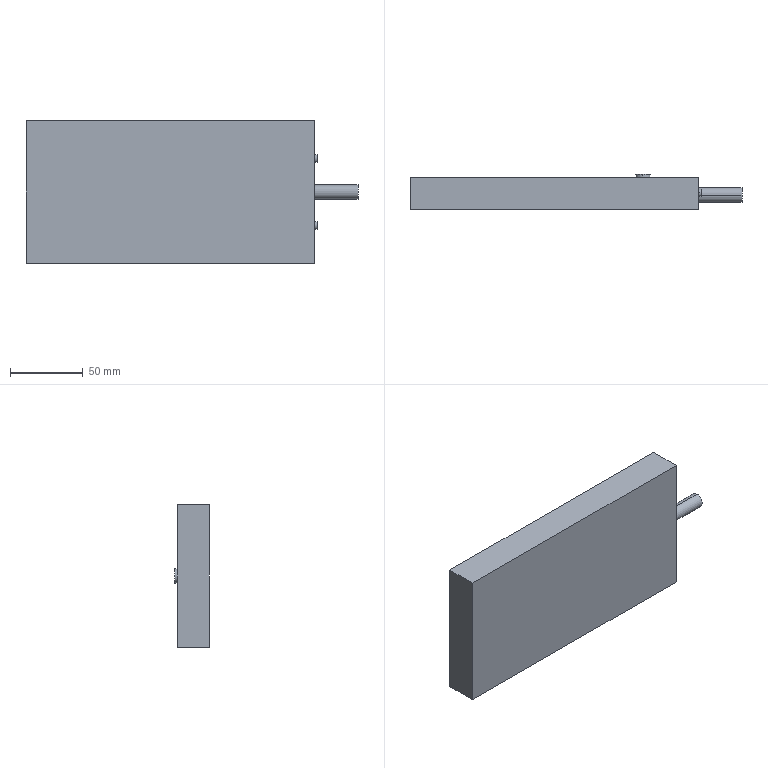Part | SolidWorks | features ICE 3, Extrusion 1 | 1 solid | 18 faces | box 228 x 24 x 98 mm | volume 429480 mm3 | plane 10 | cylinder 8 | commonest cylinder face diameters 5 x4 10 x4
STEP:
#1=CARTESIAN_POINT('',(101.,11.325,20.5));
#2=VERTEX_POINT('',#1);
#3=CARTESIAN_POINT('',(101.,11.325,25.5));
#4=VERTEX_POINT('',#3);
#5=CARTESIAN_POINT('',(101.,11.325,23.));
#6=DIRECTION('',(1.,0.,0.));
#7=DIRECTION('',(0.,0.,-1.));
#8=AXIS2_PLACEMENT_3D('',#5,#6,#7);
#9=CIRCLE('',#8,2.5);
#10=EDGE_CURVE('',#2,#4,#9,.T.);
#11=ORIENTED_EDGE('',*,*,#10,.F.);
#12=CARTESIAN_POINT('',(99.,11.325,20.5));
#13=VERTEX_POINT('',#12);
#14=CARTESIAN_POINT('',(101.,11.325,20.5));
#15=DIRECTION('',(-1.,0.,0.));
#16=VECTOR('',#15,1000.);
#17=LINE('',#14,#16);
#18=EDGE_CURVE('',#2,#13,#17,.T.);
#19=ORIENTED_EDGE('',*,*,#18,.T.);
#20=CARTESIAN_POINT('',(99.,11.325,25.5));
#21=VERTEX_POINT('',#20);
#22=CARTESIAN_POINT('',(99.,11.325,23.));
#23=DIRECTION('',(1.,0.,0.));
#24=DIRECTION('',(0.,0.,1.));
#25=AXIS2_PLACEMENT_3D('',#22,#23,#24);
#26=CIRCLE('',#25,2.5);
#27=EDGE_CURVE('',#13,#21,#26,.T.);
#28=ORIENTED_EDGE('',*,*,#27,.T.);
#29=CARTESIAN_POINT('',(101.,11.325,25.5));
#30=DIRECTION('',(-1.,0.,0.));
#31=VECTOR('',#30,1000.);
#32=LINE('',#29,#31);
#33=EDGE_CURVE('',#4,#21,#32,.T.);
#34=ORIENTED_EDGE('',*,*,#33,.F.);
#35=EDGE_LOOP('',(#11,#19,#28,#34));
#36=FACE_OUTER_BOUND('',#35,.T.);
#37=CARTESIAN_POINT('',(101.,11.325,23.));
#38=DIRECTION('',(-1.,0.,0.));
#39=DIRECTION('',(0.,0.,1.));
#40=AXIS2_PLACEMENT_3D('',#37,#38,#39);
#41=CYLINDRICAL_SURFACE('',#40,2.5);
#42=ADVANCED_FACE('',(#36),#41,.T.);
#43=CARTESIAN_POINT('',(101.,10.331,-25.5));
#44=VERTEX_POINT('',#43);
#45=CARTESIAN_POINT('',(101.,10.331,-20.5));
#46=VERTEX_POINT('',#45);
#47=CARTESIAN_POINT('',(101.,10.331,-23.));
#48=DIRECTION('',(1.,0.,0.));
#49=DIRECTION('',(0.,0.,-1.));
#50=AXIS2_PLACEMENT_3D('',#47,#48,#49);
#51=CIRCLE('',#50,2.5);
#52=EDGE_CURVE('',#44,#46,#51,.T.);
#53=ORIENTED_EDGE('',*,*,#52,.F.);
#54=CARTESIAN_POINT('',(99.,10.331,-25.5));
#55=VERTEX_POINT('',#54);
#56=CARTESIAN_POINT('',(101.,10.331,-25.5));
#57=DIRECTION('',(-1.,0.,0.));
#58=VECTOR('',#57,1000.);
#59=LINE('',#56,#58);
#60=EDGE_CURVE('',#44,#55,#59,.T.);
#61=ORIENTED_EDGE('',*,*,#60,.T.);
#62=CARTESIAN_POINT('',(99.,10.331,-20.5));
#63=VERTEX_POINT('',#62);
#64=CARTESIAN_POINT('',(99.,10.331,-23.));
#65=DIRECTION('',(1.,0.,0.));
#66=DIRECTION('',(0.,0.,1.));
#67=AXIS2_PLACEMENT_3D('',#64,#65,#66);
#68=CIRCLE('',#67,2.5);
#69=EDGE_CURVE('',#55,#63,#68,.T.);
#70=ORIENTED_EDGE('',*,*,#69,.T.);
#71=CARTESIAN_POINT('',(101.,10.331,-20.5));
#72=DIRECTION('',(-1.,0.,0.));
#73=VECTOR('',#72,1000.);
#74=LINE('',#71,#73);
#75=EDGE_CURVE('',#46,#63,#74,.T.);
#76=ORIENTED_EDGE('',*,*,#75,.F.);
#77=EDGE_LOOP('',(#53,#61,#70,#76));
#78=FACE_OUTER_BOUND('',#77,.T.);
#79=CARTESIAN_POINT('',(101.,10.331,-23.));
#80=DIRECTION('',(-1.,0.,0.));
#81=DIRECTION('',(0.,0.,1.));
#82=AXIS2_PLACEMENT_3D('',#79,#80,#81);
#83=CYLINDRICAL_SURFACE('',#82,2.5);
#84=ADVANCED_FACE('',(#78),#83,.T.);
#85=CARTESIAN_POINT('',(61.,24.,5.));
#86=VERTEX_POINT('',#85);
#87=CARTESIAN_POINT('',(61.,24.,-5.));
#88=VERTEX_POINT('',#87);
#89=CARTESIAN_POINT('',(61.,24.,0.));
#90=DIRECTION('',(0.,1.,0.));
#91=DIRECTION('',(0.,0.,1.));
#92=AXIS2_PLACEMENT_3D('',#89,#90,#91);
#93=CIRCLE('',#92,5.);
#94=EDGE_CURVE('',#86,#88,#93,.T.);
#95=ORIENTED_EDGE('',*,*,#94,.F.);
#96=CARTESIAN_POINT('',(61.,22.,5.));
#97=VERTEX_POINT('',#96);
#98=CARTESIAN_POINT('',(61.,24.,5.));
#99=DIRECTION('',(0.,-1.,0.));
#100=VECTOR('',#99,1000.);
#101=LINE('',#98,#100);
#102=EDGE_CURVE('',#86,#97,#101,.T.);
#103=ORIENTED_EDGE('',*,*,#102,.T.);
#104=CARTESIAN_POINT('',(61.,22.,-5.));
#105=VERTEX_POINT('',#104);
#106=CARTESIAN_POINT('',(61.,22.,0.));
#107=DIRECTION('',(0.,1.,0.));
#108=DIRECTION('',(0.,0.,-1.));
#109=AXIS2_PLACEMENT_3D('',#106,#107,#108);
#110=CIRCLE('',#109,5.);
#111=EDGE_CURVE('',#97,#105,#110,.T.);
#112=ORIENTED_EDGE('',*,*,#111,.T.);
#113=CARTESIAN_POINT('',(61.,24.,-5.));
#114=DIRECTION('',(0.,-1.,0.));
#115=VECTOR('',#114,1000.);
#116=LINE('',#113,#115);
#117=EDGE_CURVE('',#88,#105,#116,.T.);
#118=ORIENTED_EDGE('',*,*,#117,.F.);
#119=EDGE_LOOP('',(#95,#103,#112,#118));
#120=FACE_OUTER_BOUND('',#119,.T.);
#121=CARTESIAN_POINT('',(61.,24.,0.));
#122=DIRECTION('',(0.,-1.,0.));
#123=DIRECTION('',(0.,0.,-1.));
#124=AXIS2_PLACEMENT_3D('',#121,#122,#123);
#125=CYLINDRICAL_SURFACE('',#124,5.);
#126=ADVANCED_FACE('',(#120),#125,.T.);
#127=CARTESIAN_POINT('',(129.,9.76,-5.));
#128=VERTEX_POINT('',#127);
#129=CARTESIAN_POINT('',(129.,9.76,5.));
#130=VERTEX_POINT('',#129);
#131=CARTESIAN_POINT('',(129.,9.76,0.));
#132=DIRECTION('',(1.,0.,0.));
#133=DIRECTION('',(0.,0.,-1.));
#134=AXIS2_PLACEMENT_3D('',#131,#132,#133);
#135=CIRCLE('',#134,5.);
#136=EDGE_CURVE('',#128,#130,#135,.T.);
#137=ORIENTED_EDGE('',*,*,#136,.F.);
#138=CARTESIAN_POINT('',(99.,9.76,-5.));
#139=VERTEX_POINT('',#138);
#140=CARTESIAN_POINT('',(129.,9.76,-5.));
#141=DIRECTION('',(-1.,0.,0.));
#142=VECTOR('',#141,1000.);
#143=LINE('',#140,#142);
#144=EDGE_CURVE('',#128,#139,#143,.T.);
#145=ORIENTED_EDGE('',*,*,#144,.T.);
#146=CARTESIAN_POINT('',(99.,9.76,5.));
#147=VERTEX_POINT('',#146);
#148=CARTESIAN_POINT('',(99.,9.76,0.));
#149=DIRECTION('',(1.,0.,0.));
#150=DIRECTION('',(0.,0.,1.));
#151=AXIS2_PLACEMENT_3D('',#148,#149,#150);
#152=CIRCLE('',#151,5.);
#153=EDGE_CURVE('',#139,#147,#152,.T.);
#154=ORIENTED_EDGE('',*,*,#153,.T.);
#155=CARTESIAN_POINT('',(129.,9.76,5.));
#156=DIRECTION('',(-1.,0.,0.));
#157=VECTOR('',#156,1000.);
#158=LINE('',#155,#157);
#159=EDGE_CURVE('',#130,#147,#158,.T.);
#160=ORIENTED_EDGE('',*,*,#159,.F.);
#161=EDGE_LOOP('',(#137,#145,#154,#160));
#162=FACE_OUTER_BOUND('',#161,.T.);
#163=CARTESIAN_POINT('',(129.,9.76,0.));
#164=DIRECTION('',(-1.,0.,0.));
#165=DIRECTION('',(0.,0.,1.));
#166=AXIS2_PLACEMENT_3D('',#163,#164,#165);
#167=CYLINDRICAL_SURFACE('',#166,5.);
#168=ADVANCED_FACE('',(#162),#167,.T.);
#169=CARTESIAN_POINT('',(99.,11.325,23.));
#170=DIRECTION('',(1.,0.,0.));
#171=DIRECTION('',(0.,0.,1.));
#172=AXIS2_PLACEMENT_3D('',#169,#170,#171);
#173=CIRCLE('',#172,2.5);
#174=EDGE_CURVE('',#21,#13,#173,.T.);
#175=ORIENTED_EDGE('',*,*,#174,.F.);
#176=ORIENTED_EDGE('',*,*,#27,.F.);
#177=EDGE_LOOP('',(#175,#176));
#178=FACE_BOUND('',#177,.T.);
#179=CARTESIAN_POINT('',(99.,10.331,-23.));
#180=DIRECTION('',(1.,0.,0.));
#181=DIRECTION('',(0.,0.,1.));
#182=AXIS2_PLACEMENT_3D('',#179,#180,#181);
#183=CIRCLE('',#182,2.5);
#184=EDGE_CURVE('',#63,#55,#183,.T.);
#185=ORIENTED_EDGE('',*,*,#184,.F.);
#186=ORIENTED_EDGE('',*,*,#69,.F.);
#187=EDGE_LOOP('',(#185,#186));
#188=FACE_BOUND('',#187,.T.);
#189=CARTESIAN_POINT('',(99.,9.76,0.));
#190=DIRECTION('',(1.,0.,0.));
#191=DIRECTION('',(0.,0.,1.));
#192=AXIS2_PLACEMENT_3D('',#189,#190,#191);
#193=CIRCLE('',#192,5.);
#194=EDGE_CURVE('',#147,#139,#193,.T.);
#195=ORIENTED_EDGE('',*,*,#194,.F.);
#196=ORIENTED_EDGE('',*,*,#153,.F.);
#197=EDGE_LOOP('',(#195,#196));
#198=FACE_BOUND('',#197,.T.);
#199=CARTESIAN_POINT('',(99.,0.,49.));
#200=VERTEX_POINT('',#199);
#201=CARTESIAN_POINT('',(99.,0.,-49.));
#202=VERTEX_POINT('',#201);
#203=CARTESIAN_POINT('',(99.,0.,49.));
#204=DIRECTION('',(0.,0.,-1.));
#205=VECTOR('',#204,1000.);
#206=LINE('',#203,#205);
#207=EDGE_CURVE('',#200,#202,#206,.T.);
#208=ORIENTED_EDGE('',*,*,#207,.T.);
#209=CARTESIAN_POINT('',(99.,22.,-49.));
#210=VERTEX_POINT('',#209);
#211=CARTESIAN_POINT('',(99.,22.,-49.));
#212=DIRECTION('',(0.,-1.,0.));
#213=VECTOR('',#212,1000.);
#214=LINE('',#211,#213);
#215=EDGE_CURVE('',#210,#202,#214,.T.);
#216=ORIENTED_EDGE('',*,*,#215,.F.);
#217=CARTESIAN_POINT('',(99.,22.,49.));
#218=VERTEX_POINT('',#217);
#219=CARTESIAN_POINT('',(99.,22.,49.));
#220=DIRECTION('',(0.,0.,-1.));
#221=VECTOR('',#220,1000.);
#222=LINE('',#219,#221);
#223=EDGE_CURVE('',#218,#210,#222,.T.);
#224=ORIENTED_EDGE('',*,*,#223,.F.);
#225=CARTESIAN_POINT('',(99.,22.,49.));
#226=DIRECTION('',(0.,-1.,0.));
#227=VECTOR('',#226,1000.);
#228=LINE('',#225,#227);
#229=EDGE_CURVE('',#218,#200,#228,.T.);
#230=ORIENTED_EDGE('',*,*,#229,.T.);
#231=EDGE_LOOP('',(#208,#216,#224,#230));
#232=FACE_OUTER_BOUND('',#231,.T.);
#233=CARTESIAN_POINT('',(99.,22.,49.));
#234=DIRECTION('',(-1.,0.,0.));
#235=DIRECTION('',(0.,0.,1.));
#236=AXIS2_PLACEMENT_3D('',#233,#234,#235);
#237=PLANE('',#236);
#238=ADVANCED_FACE('',(#178,#188,#198,#232),#237,.F.);
#239=CARTESIAN_POINT('',(-99.,0.,-49.));
#240=VERTEX_POINT('',#239);
#241=CARTESIAN_POINT('',(-99.,0.,-49.));
#242=DIRECTION('',(-1.,0.,0.));
#243=VECTOR('',#242,1000.);
#244=LINE('',#241,#243);
#245=EDGE_CURVE('',#202,#240,#244,.T.);
#246=ORIENTED_EDGE('',*,*,#245,.T.);
#247=CARTESIAN_POINT('',(-99.,22.,-49.));
#248=VERTEX_POINT('',#247);
#249=CARTESIAN_POINT('',(-99.,22.,-49.));
#250=DIRECTION('',(0.,-1.,0.));
#251=VECTOR('',#250,1000.);
#252=LINE('',#249,#251);
#253=EDGE_CURVE('',#248,#240,#252,.T.);
#254=ORIENTED_EDGE('',*,*,#253,.F.);
#255=CARTESIAN_POINT('',(-99.,22.,-49.));
#256=DIRECTION('',(-1.,0.,0.));
#257=VECTOR('',#256,1000.);
#258=LINE('',#255,#257);
#259=EDGE_CURVE('',#210,#248,#258,.T.);
#260=ORIENTED_EDGE('',*,*,#259,.F.);
#261=ORIENTED_EDGE('',*,*,#215,.T.);
#262=EDGE_LOOP('',(#246,#254,#260,#261));
#263=FACE_OUTER_BOUND('',#262,.T.);
#264=CARTESIAN_POINT('',(-99.,22.,-49.));
#265=DIRECTION('',(0.,0.,1.));
#266=DIRECTION('',(1.,0.,0.));
#267=AXIS2_PLACEMENT_3D('',#264,#265,#266);
#268=PLANE('',#267);
#269=ADVANCED_FACE('',(#263),#268,.F.);
#270=CARTESIAN_POINT('',(-99.,0.,49.));
#271=VERTEX_POINT('',#270);
#272=CARTESIAN_POINT('',(-99.,0.,49.));
#273=DIRECTION('',(0.,0.,1.));
#274=VECTOR('',#273,1000.);
#275=LINE('',#272,#274);
#276=EDGE_CURVE('',#240,#271,#275,.T.);
#277=ORIENTED_EDGE('',*,*,#276,.T.);
#278=CARTESIAN_POINT('',(-99.,22.,49.));
#279=VERTEX_POINT('',#278);
#280=CARTESIAN_POINT('',(-99.,22.,49.));
#281=DIRECTION('',(0.,-1.,0.));
#282=VECTOR('',#281,1000.);
#283=LINE('',#280,#282);
#284=EDGE_CURVE('',#279,#271,#283,.T.);
#285=ORIENTED_EDGE('',*,*,#284,.F.);
#286=CARTESIAN_POINT('',(-99.,22.,49.));
#287=DIRECTION('',(0.,0.,1.));
#288=VECTOR('',#287,1000.);
#289=LINE('',#286,#288);
#290=EDGE_CURVE('',#248,#279,#289,.T.);
#291=ORIENTED_EDGE('',*,*,#290,.F.);
#292=ORIENTED_EDGE('',*,*,#253,.T.);
#293=EDGE_LOOP('',(#277,#285,#291,#292));
#294=FACE_OUTER_BOUND('',#293,.T.);
#295=CARTESIAN_POINT('',(-99.,22.,49.));
#296=DIRECTION('',(1.,0.,0.));
#297=DIRECTION('',(0.,0.,-1.));
#298=AXIS2_PLACEMENT_3D('',#295,#296,#297);
#299=PLANE('',#298);
#300=ADVANCED_FACE('',(#294),#299,.F.);
#301=CARTESIAN_POINT('',(-99.,0.,49.));
#302=DIRECTION('',(1.,0.,0.));
#303=VECTOR('',#302,1000.);
#304=LINE('',#301,#303);
#305=EDGE_CURVE('',#271,#200,#304,.T.);
#306=ORIENTED_EDGE('',*,*,#305,.T.);
#307=ORIENTED_EDGE('',*,*,#229,.F.);
#308=CARTESIAN_POINT('',(-99.,22.,49.));
#309=DIRECTION('',(1.,0.,0.));
#310=VECTOR('',#309,1000.);
#311=LINE('',#308,#310);
#312=EDGE_CURVE('',#279,#218,#311,.T.);
#313=ORIENTED_EDGE('',*,*,#312,.F.);
#314=ORIENTED_EDGE('',*,*,#284,.T.);
#315=EDGE_LOOP('',(#306,#307,#313,#314));
#316=FACE_OUTER_BOUND('',#315,.T.);
#317=CARTESIAN_POINT('',(-99.,22.,49.));
#318=DIRECTION('',(0.,0.,-1.));
#319=DIRECTION('',(-1.,0.,0.));
#320=AXIS2_PLACEMENT_3D('',#317,#318,#319);
#321=PLANE('',#320);
#322=ADVANCED_FACE('',(#316),#321,.F.);
#323=CARTESIAN_POINT('',(61.,22.,0.));
#324=DIRECTION('',(0.,1.,0.));
#325=DIRECTION('',(0.,0.,-1.));
#326=AXIS2_PLACEMENT_3D('',#323,#324,#325);
#327=CIRCLE('',#326,5.);
#328=EDGE_CURVE('',#105,#97,#327,.T.);
#329=ORIENTED_EDGE('',*,*,#328,.F.);
#330=ORIENTED_EDGE('',*,*,#111,.F.);
#331=EDGE_LOOP('',(#329,#330));
#332=FACE_BOUND('',#331,.T.);
#333=ORIENTED_EDGE('',*,*,#223,.T.);
#334=ORIENTED_EDGE('',*,*,#259,.T.);
#335=ORIENTED_EDGE('',*,*,#290,.T.);
#336=ORIENTED_EDGE('',*,*,#312,.T.);
#337=EDGE_LOOP('',(#333,#334,#335,#336));
#338=FACE_OUTER_BOUND('',#337,.T.);
#339=CARTESIAN_POINT('',(0.,22.,0.));
#340=DIRECTION('',(0.,-1.,0.));
#341=DIRECTION('',(0.,0.,-1.));
#342=AXIS2_PLACEMENT_3D('',#339,#340,#341);
#343=PLANE('',#342);
#344=ADVANCED_FACE('',(#332,#338),#343,.F.);
#345=ORIENTED_EDGE('',*,*,#207,.F.);
#346=ORIENTED_EDGE('',*,*,#305,.F.);
#347=ORIENTED_EDGE('',*,*,#276,.F.);
#348=ORIENTED_EDGE('',*,*,#245,.F.);
#349=EDGE_LOOP('',(#345,#346,#347,#348));
#350=FACE_OUTER_BOUND('',#349,.T.);
#351=CARTESIAN_POINT('',(0.,0.,0.));
#352=DIRECTION('',(0.,-1.,0.));
#353=DIRECTION('',(0.,0.,-1.));
#354=AXIS2_PLACEMENT_3D('',#351,#352,#353);
#355=PLANE('',#354);
#356=ADVANCED_FACE('',(#350),#355,.T.);
#357=ORIENTED_EDGE('',*,*,#144,.F.);
#358=CARTESIAN_POINT('',(129.,9.76,0.));
#359=DIRECTION('',(1.,0.,0.));
#360=DIRECTION('',(0.,0.,-1.));
#361=AXIS2_PLACEMENT_3D('',#358,#359,#360);
#362=CIRCLE('',#361,5.);
#363=EDGE_CURVE('',#130,#128,#362,.T.);
#364=ORIENTED_EDGE('',*,*,#363,.F.);
#365=ORIENTED_EDGE('',*,*,#159,.T.);
#366=ORIENTED_EDGE('',*,*,#194,.T.);
#367=EDGE_LOOP('',(#357,#364,#365,#366));
#368=FACE_OUTER_BOUND('',#367,.T.);
#369=CARTESIAN_POINT('',(129.,9.76,0.));
#370=DIRECTION('',(-1.,0.,0.));
#371=DIRECTION('',(0.,0.,1.));
#372=AXIS2_PLACEMENT_3D('',#369,#370,#371);
#373=CYLINDRICAL_SURFACE('',#372,5.);
#374=ADVANCED_FACE('',(#368),#373,.T.);
#375=ORIENTED_EDGE('',*,*,#363,.T.);
#376=ORIENTED_EDGE('',*,*,#136,.T.);
#377=EDGE_LOOP('',(#375,#376));
#378=FACE_OUTER_BOUND('',#377,.T.);
#379=CARTESIAN_POINT('',(129.,9.76,0.));
#380=DIRECTION('',(1.,0.,0.));
#381=DIRECTION('',(0.,0.,-1.));
#382=AXIS2_PLACEMENT_3D('',#379,#380,#381);
#383=PLANE('',#382);
#384=ADVANCED_FACE('',(#378),#383,.T.);
#385=ORIENTED_EDGE('',*,*,#102,.F.);
#386=CARTESIAN_POINT('',(61.,24.,0.));
#387=DIRECTION('',(0.,1.,0.));
#388=DIRECTION('',(0.,0.,1.));
#389=AXIS2_PLACEMENT_3D('',#386,#387,#388);
#390=CIRCLE('',#389,5.);
#391=EDGE_CURVE('',#88,#86,#390,.T.);
#392=ORIENTED_EDGE('',*,*,#391,.F.);
#393=ORIENTED_EDGE('',*,*,#117,.T.);
#394=ORIENTED_EDGE('',*,*,#328,.T.);
#395=EDGE_LOOP('',(#385,#392,#393,#394));
#396=FACE_OUTER_BOUND('',#395,.T.);
#397=CARTESIAN_POINT('',(61.,24.,0.));
#398=DIRECTION('',(0.,-1.,0.));
#399=DIRECTION('',(0.,0.,-1.));
#400=AXIS2_PLACEMENT_3D('',#397,#398,#399);
#401=CYLINDRICAL_SURFACE('',#400,5.);
#402=ADVANCED_FACE('',(#396),#401,.T.);
#403=ORIENTED_EDGE('',*,*,#391,.T.);
#404=ORIENTED_EDGE('',*,*,#94,.T.);
#405=EDGE_LOOP('',(#403,#404));
#406=FACE_OUTER_BOUND('',#405,.T.);
#407=CARTESIAN_POINT('',(61.,24.,0.));
#408=DIRECTION('',(0.,1.,0.));
#409=DIRECTION('',(0.,0.,1.));
#410=AXIS2_PLACEMENT_3D('',#407,#408,#409);
#411=PLANE('',#410);
#412=ADVANCED_FACE('',(#406),#411,.T.);
#413=ORIENTED_EDGE('',*,*,#60,.F.);
#414=CARTESIAN_POINT('',(101.,10.331,-23.));
#415=DIRECTION('',(1.,0.,0.));
#416=DIRECTION('',(0.,0.,-1.));
#417=AXIS2_PLACEMENT_3D('',#414,#415,#416);
#418=CIRCLE('',#417,2.5);
#419=EDGE_CURVE('',#46,#44,#418,.T.);
#420=ORIENTED_EDGE('',*,*,#419,.F.);
#421=ORIENTED_EDGE('',*,*,#75,.T.);
#422=ORIENTED_EDGE('',*,*,#184,.T.);
#423=EDGE_LOOP('',(#413,#420,#421,#422));
#424=FACE_OUTER_BOUND('',#423,.T.);
#425=CARTESIAN_POINT('',(101.,10.331,-23.));
#426=DIRECTION('',(-1.,0.,0.));
#427=DIRECTION('',(0.,0.,1.));
#428=AXIS2_PLACEMENT_3D('',#425,#426,#427);
#429=CYLINDRICAL_SURFACE('',#428,2.5);
#430=ADVANCED_FACE('',(#424),#429,.T.);
#431=ORIENTED_EDGE('',*,*,#419,.T.);
#432=ORIENTED_EDGE('',*,*,#52,.T.);
#433=EDGE_LOOP('',(#431,#432));
#434=FACE_OUTER_BOUND('',#433,.T.);
#435=CARTESIAN_POINT('',(101.,10.331,-23.));
#436=DIRECTION('',(1.,0.,0.));
#437=DIRECTION('',(0.,0.,-1.));
#438=AXIS2_PLACEMENT_3D('',#435,#436,#437);
#439=PLANE('',#438);
#440=ADVANCED_FACE('',(#434),#439,.T.);
#441=ORIENTED_EDGE('',*,*,#18,.F.);
#442=CARTESIAN_POINT('',(101.,11.325,23.));
#443=DIRECTION('',(1.,0.,0.));
#444=DIRECTION('',(0.,0.,-1.));
#445=AXIS2_PLACEMENT_3D('',#442,#443,#444);
#446=CIRCLE('',#445,2.5);
#447=EDGE_CURVE('',#4,#2,#446,.T.);
#448=ORIENTED_EDGE('',*,*,#447,.F.);
#449=ORIENTED_EDGE('',*,*,#33,.T.);
#450=ORIENTED_EDGE('',*,*,#174,.T.);
#451=EDGE_LOOP('',(#441,#448,#449,#450));
#452=FACE_OUTER_BOUND('',#451,.T.);
#453=CARTESIAN_POINT('',(101.,11.325,23.));
#454=DIRECTION('',(-1.,0.,0.));
#455=DIRECTION('',(0.,0.,1.));
#456=AXIS2_PLACEMENT_3D('',#453,#454,#455);
#457=CYLINDRICAL_SURFACE('',#456,2.5);
#458=ADVANCED_FACE('',(#452),#457,.T.);
#459=ORIENTED_EDGE('',*,*,#447,.T.);
#460=ORIENTED_EDGE('',*,*,#10,.T.);
#461=EDGE_LOOP('',(#459,#460));
#462=FACE_OUTER_BOUND('',#461,.T.);
#463=CARTESIAN_POINT('',(101.,11.325,23.));
#464=DIRECTION('',(1.,0.,0.));
#465=DIRECTION('',(0.,0.,-1.));
#466=AXIS2_PLACEMENT_3D('',#463,#464,#465);
#467=PLANE('',#466);
#468=ADVANCED_FACE('',(#462),#467,.T.);
#469=CLOSED_SHELL('',(#42,#84,#126,#168,#238,#269,#300,#322,#344,#356,#374,#384,#402,#412,#430,#440,#458,#468));
#470=MANIFOLD_SOLID_BREP('',#469);
#471=CARTESIAN_POINT('',(0.,0.,0.));
#472=DIRECTION('',(0.,0.,1.));
#473=DIRECTION('',(1.,0.,0.));
#474=AXIS2_PLACEMENT_3D('',#471,#472,#473);
#475=(LENGTH_UNIT()NAMED_UNIT(*)SI_UNIT(.MILLI.,.METRE.));
#476=UNCERTAINTY_MEASURE_WITH_UNIT(LENGTH_MEASURE(0.00001),#475,'','');
#477=(NAMED_UNIT(*)PLANE_ANGLE_UNIT()SI_UNIT($,.RADIAN.));
#478=(NAMED_UNIT(*)SI_UNIT($,.STERADIAN.)SOLID_ANGLE_UNIT());
#479=(GEOMETRIC_REPRESENTATION_CONTEXT(3)GLOBAL_UNCERTAINTY_ASSIGNED_CONTEXT((#476))GLOBAL_UNIT_ASSIGNED_CONTEXT((#475,#477,#478))REPRESENTATION_CONTEXT('',''));
#480=ADVANCED_BREP_SHAPE_REPRESENTATION('',(#470,#474),#479);